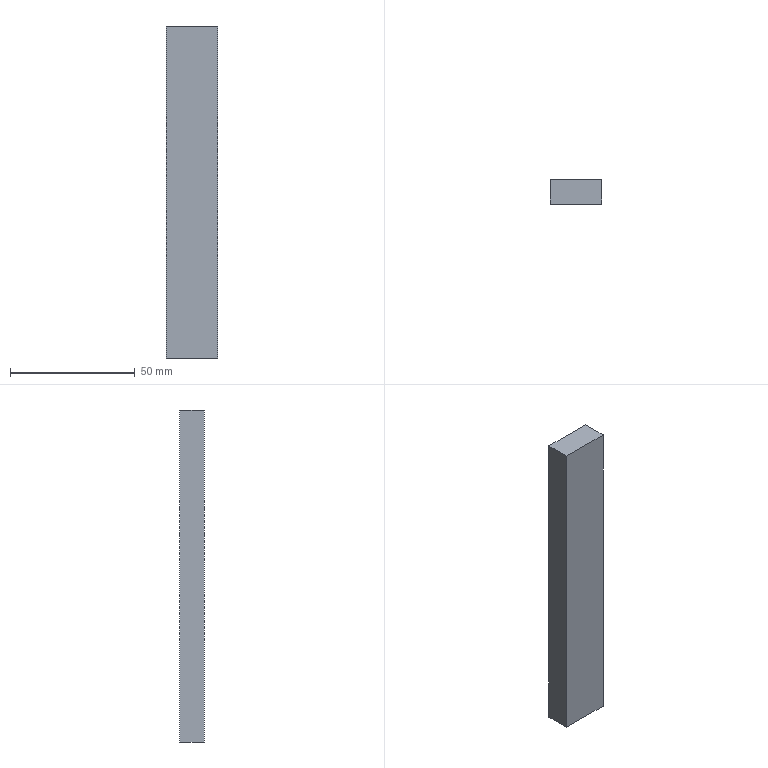Part | STEP file | 1 solid | 6 faces | box 20.737 x 10 x 133 mm | volume 27580 mm3 | plane 6
STEP:
#1=CARTESIAN_POINT('',(0.,0.,0.));
#2=DIRECTION('',(0.,0.,1.));
#3=DIRECTION('',(1.,0.,0.));
#4=AXIS2_PLACEMENT_3D('',#1,#2,#3);
#5=CARTESIAN_POINT('',(-23.708,79.267,216.926));
#6=VERTEX_POINT('',#5);
#7=CARTESIAN_POINT('',(-23.708,79.267,349.926));
#8=VERTEX_POINT('',#7);
#9=CARTESIAN_POINT('',(-23.708,79.267,216.926));
#10=DIRECTION('',(0.,0.,1.));
#11=VECTOR('',#10,1.);
#12=LINE('',#9,#11);
#13=CARTESIAN_POINT('',(-23.708,89.267,216.926));
#14=DIRECTION('',(1.,0.,0.));
#15=DIRECTION('',(0.,1.,0.));
#16=AXIS2_PLACEMENT_3D('',#13,#14,#15);
#17=PLANE('',#16);
#18=CARTESIAN_POINT('',(-10.,0.));
#19=DIRECTION('',(0.,1.));
#20=VECTOR('',#19,1.);
#21=LINE('',#18,#20);
#22=(GEOMETRIC_REPRESENTATION_CONTEXT(2)PARAMETRIC_REPRESENTATION_CONTEXT()REPRESENTATION_CONTEXT('',''));
#23=DEFINITIONAL_REPRESENTATION('',(#21),#22);
#24=PCURVE('',#17,#23);
#25=CARTESIAN_POINT('',(0.,79.267,0.));
#26=DIRECTION('',(0.,1.,0.));
#27=DIRECTION('',(0.,0.,1.));
#28=AXIS2_PLACEMENT_3D('',#25,#26,#27);
#29=PLANE('',#28);
#30=CARTESIAN_POINT('',(216.926,-23.708));
#31=DIRECTION('',(1.,0.));
#32=VECTOR('',#31,1.);
#33=LINE('',#30,#32);
#34=(GEOMETRIC_REPRESENTATION_CONTEXT(2)PARAMETRIC_REPRESENTATION_CONTEXT()REPRESENTATION_CONTEXT('',''));
#35=DEFINITIONAL_REPRESENTATION('',(#33),#34);
#36=PCURVE('',#29,#35);
#37=SURFACE_CURVE('',#12,(#24,#36),.PCURVE_S1.);
#38=EDGE_CURVE('',#6,#8,#37,.T.);
#39=ORIENTED_EDGE('',*,*,#38,.T.);
#40=CARTESIAN_POINT('',(-23.708,89.267,349.926));
#41=VERTEX_POINT('',#40);
#42=CARTESIAN_POINT('',(-23.708,89.267,349.926));
#43=DIRECTION('',(0.,-1.,0.));
#44=VECTOR('',#43,1.);
#45=LINE('',#42,#44);
#46=CARTESIAN_POINT('',(0.,133.));
#47=DIRECTION('',(-1.,0.));
#48=VECTOR('',#47,1.);
#49=LINE('',#46,#48);
#50=(GEOMETRIC_REPRESENTATION_CONTEXT(2)PARAMETRIC_REPRESENTATION_CONTEXT()REPRESENTATION_CONTEXT('',''));
#51=DEFINITIONAL_REPRESENTATION('',(#49),#50);
#52=PCURVE('',#17,#51);
#53=CARTESIAN_POINT('',(-23.708,89.267,349.926));
#54=DIRECTION('',(0.,0.,-1.));
#55=DIRECTION('',(-1.,0.,0.));
#56=AXIS2_PLACEMENT_3D('',#53,#54,#55);
#57=PLANE('',#56);
#58=CARTESIAN_POINT('',(0.,0.));
#59=DIRECTION('',(0.,-1.));
#60=VECTOR('',#59,1.);
#61=LINE('',#58,#60);
#62=(GEOMETRIC_REPRESENTATION_CONTEXT(2)PARAMETRIC_REPRESENTATION_CONTEXT()REPRESENTATION_CONTEXT('',''));
#63=DEFINITIONAL_REPRESENTATION('',(#61),#62);
#64=PCURVE('',#57,#63);
#65=SURFACE_CURVE('',#45,(#52,#64),.PCURVE_S1.);
#66=EDGE_CURVE('',#41,#8,#65,.T.);
#67=ORIENTED_EDGE('',*,*,#66,.F.);
#68=CARTESIAN_POINT('',(-23.708,89.267,216.926));
#69=VERTEX_POINT('',#68);
#70=CARTESIAN_POINT('',(-23.708,89.267,216.926));
#71=DIRECTION('',(0.,0.,1.));
#72=VECTOR('',#71,1.);
#73=LINE('',#70,#72);
#74=CARTESIAN_POINT('',(0.,0.));
#75=DIRECTION('',(0.,1.));
#76=VECTOR('',#75,1.);
#77=LINE('',#74,#76);
#78=(GEOMETRIC_REPRESENTATION_CONTEXT(2)PARAMETRIC_REPRESENTATION_CONTEXT()REPRESENTATION_CONTEXT('',''));
#79=DEFINITIONAL_REPRESENTATION('',(#77),#78);
#80=PCURVE('',#17,#79);
#81=CARTESIAN_POINT('',(0.,89.267,0.));
#82=DIRECTION('',(0.,1.,0.));
#83=DIRECTION('',(0.,0.,1.));
#84=AXIS2_PLACEMENT_3D('',#81,#82,#83);
#85=PLANE('',#84);
#86=CARTESIAN_POINT('',(216.926,-23.708));
#87=DIRECTION('',(1.,0.));
#88=VECTOR('',#87,1.);
#89=LINE('',#86,#88);
#90=(GEOMETRIC_REPRESENTATION_CONTEXT(2)PARAMETRIC_REPRESENTATION_CONTEXT()REPRESENTATION_CONTEXT('',''));
#91=DEFINITIONAL_REPRESENTATION('',(#89),#90);
#92=PCURVE('',#85,#91);
#93=SURFACE_CURVE('',#73,(#80,#92),.PCURVE_S1.);
#94=EDGE_CURVE('',#69,#41,#93,.T.);
#95=ORIENTED_EDGE('',*,*,#94,.F.);
#96=CARTESIAN_POINT('',(-23.708,89.267,216.926));
#97=DIRECTION('',(0.,-1.,0.));
#98=VECTOR('',#97,1.);
#99=LINE('',#96,#98);
#100=CARTESIAN_POINT('',(0.,0.));
#101=DIRECTION('',(-1.,0.));
#102=VECTOR('',#101,1.);
#103=LINE('',#100,#102);
#104=(GEOMETRIC_REPRESENTATION_CONTEXT(2)PARAMETRIC_REPRESENTATION_CONTEXT()REPRESENTATION_CONTEXT('',''));
#105=DEFINITIONAL_REPRESENTATION('',(#103),#104);
#106=PCURVE('',#17,#105);
#107=CARTESIAN_POINT('',(-23.708,89.267,216.926));
#108=DIRECTION('',(0.,0.,1.));
#109=DIRECTION('',(1.,0.,0.));
#110=AXIS2_PLACEMENT_3D('',#107,#108,#109);
#111=PLANE('',#110);
#112=CARTESIAN_POINT('',(0.,0.));
#113=DIRECTION('',(0.,-1.));
#114=VECTOR('',#113,1.);
#115=LINE('',#112,#114);
#116=(GEOMETRIC_REPRESENTATION_CONTEXT(2)PARAMETRIC_REPRESENTATION_CONTEXT()REPRESENTATION_CONTEXT('',''));
#117=DEFINITIONAL_REPRESENTATION('',(#115),#116);
#118=PCURVE('',#111,#117);
#119=SURFACE_CURVE('',#99,(#106,#118),.PCURVE_S1.);
#120=EDGE_CURVE('',#69,#6,#119,.T.);
#121=ORIENTED_EDGE('',*,*,#120,.T.);
#122=EDGE_LOOP('',(#39,#67,#95,#121));
#123=FACE_BOUND('',#122,.T.);
#124=ADVANCED_FACE('',(#123),#17,.F.);
#125=CARTESIAN_POINT('',(-2.971,79.267,349.926));
#126=VERTEX_POINT('',#125);
#127=CARTESIAN_POINT('',(-23.708,79.267,349.926));
#128=DIRECTION('',(1.,0.,0.));
#129=VECTOR('',#128,1.);
#130=LINE('',#127,#129);
#131=CARTESIAN_POINT('',(0.,-10.));
#132=DIRECTION('',(-1.,0.));
#133=VECTOR('',#132,1.);
#134=LINE('',#131,#133);
#135=(GEOMETRIC_REPRESENTATION_CONTEXT(2)PARAMETRIC_REPRESENTATION_CONTEXT()REPRESENTATION_CONTEXT('',''));
#136=DEFINITIONAL_REPRESENTATION('',(#134),#135);
#137=PCURVE('',#57,#136);
#138=CARTESIAN_POINT('',(349.926,-23.708));
#139=DIRECTION('',(0.,1.));
#140=VECTOR('',#139,1.);
#141=LINE('',#138,#140);
#142=(GEOMETRIC_REPRESENTATION_CONTEXT(2)PARAMETRIC_REPRESENTATION_CONTEXT()REPRESENTATION_CONTEXT('',''));
#143=DEFINITIONAL_REPRESENTATION('',(#141),#142);
#144=PCURVE('',#29,#143);
#145=SURFACE_CURVE('',#130,(#137,#144),.PCURVE_S1.);
#146=EDGE_CURVE('',#8,#126,#145,.T.);
#147=ORIENTED_EDGE('',*,*,#146,.T.);
#148=CARTESIAN_POINT('',(-2.971,89.267,349.926));
#149=VERTEX_POINT('',#148);
#150=CARTESIAN_POINT('',(-2.971,89.267,349.926));
#151=DIRECTION('',(0.,-1.,0.));
#152=VECTOR('',#151,1.);
#153=LINE('',#150,#152);
#154=CARTESIAN_POINT('',(-20.737,0.));
#155=DIRECTION('',(0.,-1.));
#156=VECTOR('',#155,1.);
#157=LINE('',#154,#156);
#158=(GEOMETRIC_REPRESENTATION_CONTEXT(2)PARAMETRIC_REPRESENTATION_CONTEXT()REPRESENTATION_CONTEXT('',''));
#159=DEFINITIONAL_REPRESENTATION('',(#157),#158);
#160=PCURVE('',#57,#159);
#161=CARTESIAN_POINT('',(-2.971,89.267,216.926));
#162=DIRECTION('',(-1.,0.,0.));
#163=DIRECTION('',(0.,0.,1.));
#164=AXIS2_PLACEMENT_3D('',#161,#162,#163);
#165=PLANE('',#164);
#166=CARTESIAN_POINT('',(133.,0.));
#167=DIRECTION('',(0.,-1.));
#168=VECTOR('',#167,1.);
#169=LINE('',#166,#168);
#170=(GEOMETRIC_REPRESENTATION_CONTEXT(2)PARAMETRIC_REPRESENTATION_CONTEXT()REPRESENTATION_CONTEXT('',''));
#171=DEFINITIONAL_REPRESENTATION('',(#169),#170);
#172=PCURVE('',#165,#171);
#173=SURFACE_CURVE('',#153,(#160,#172),.PCURVE_S1.);
#174=EDGE_CURVE('',#149,#126,#173,.T.);
#175=ORIENTED_EDGE('',*,*,#174,.F.);
#176=CARTESIAN_POINT('',(-23.708,89.267,349.926));
#177=DIRECTION('',(1.,0.,0.));
#178=VECTOR('',#177,1.);
#179=LINE('',#176,#178);
#180=CARTESIAN_POINT('',(0.,0.));
#181=DIRECTION('',(-1.,0.));
#182=VECTOR('',#181,1.);
#183=LINE('',#180,#182);
#184=(GEOMETRIC_REPRESENTATION_CONTEXT(2)PARAMETRIC_REPRESENTATION_CONTEXT()REPRESENTATION_CONTEXT('',''));
#185=DEFINITIONAL_REPRESENTATION('',(#183),#184);
#186=PCURVE('',#57,#185);
#187=CARTESIAN_POINT('',(349.926,-23.708));
#188=DIRECTION('',(0.,1.));
#189=VECTOR('',#188,1.);
#190=LINE('',#187,#189);
#191=(GEOMETRIC_REPRESENTATION_CONTEXT(2)PARAMETRIC_REPRESENTATION_CONTEXT()REPRESENTATION_CONTEXT('',''));
#192=DEFINITIONAL_REPRESENTATION('',(#190),#191);
#193=PCURVE('',#85,#192);
#194=SURFACE_CURVE('',#179,(#186,#193),.PCURVE_S1.);
#195=EDGE_CURVE('',#41,#149,#194,.T.);
#196=ORIENTED_EDGE('',*,*,#195,.F.);
#197=ORIENTED_EDGE('',*,*,#66,.T.);
#198=EDGE_LOOP('',(#147,#175,#196,#197));
#199=FACE_BOUND('',#198,.T.);
#200=ADVANCED_FACE('',(#199),#57,.F.);
#201=CARTESIAN_POINT('',(-2.971,79.267,216.926));
#202=VERTEX_POINT('',#201);
#203=CARTESIAN_POINT('',(-2.971,79.267,216.926));
#204=DIRECTION('',(0.,0.,-1.));
#205=VECTOR('',#204,1.);
#206=LINE('',#203,#205);
#207=CARTESIAN_POINT('',(0.,-10.));
#208=DIRECTION('',(-1.,0.));
#209=VECTOR('',#208,1.);
#210=LINE('',#207,#209);
#211=(GEOMETRIC_REPRESENTATION_CONTEXT(2)PARAMETRIC_REPRESENTATION_CONTEXT()REPRESENTATION_CONTEXT('',''));
#212=DEFINITIONAL_REPRESENTATION('',(#210),#211);
#213=PCURVE('',#165,#212);
#214=CARTESIAN_POINT('',(216.926,-2.971));
#215=DIRECTION('',(-1.,0.));
#216=VECTOR('',#215,1.);
#217=LINE('',#214,#216);
#218=(GEOMETRIC_REPRESENTATION_CONTEXT(2)PARAMETRIC_REPRESENTATION_CONTEXT()REPRESENTATION_CONTEXT('',''));
#219=DEFINITIONAL_REPRESENTATION('',(#217),#218);
#220=PCURVE('',#29,#219);
#221=SURFACE_CURVE('',#206,(#213,#220),.PCURVE_S1.);
#222=EDGE_CURVE('',#126,#202,#221,.T.);
#223=ORIENTED_EDGE('',*,*,#222,.T.);
#224=CARTESIAN_POINT('',(-2.971,89.267,216.926));
#225=VERTEX_POINT('',#224);
#226=CARTESIAN_POINT('',(-2.971,89.267,216.926));
#227=DIRECTION('',(0.,-1.,0.));
#228=VECTOR('',#227,1.);
#229=LINE('',#226,#228);
#230=CARTESIAN_POINT('',(0.,0.));
#231=DIRECTION('',(0.,-1.));
#232=VECTOR('',#231,1.);
#233=LINE('',#230,#232);
#234=(GEOMETRIC_REPRESENTATION_CONTEXT(2)PARAMETRIC_REPRESENTATION_CONTEXT()REPRESENTATION_CONTEXT('',''));
#235=DEFINITIONAL_REPRESENTATION('',(#233),#234);
#236=PCURVE('',#165,#235);
#237=CARTESIAN_POINT('',(20.737,0.));
#238=DIRECTION('',(0.,-1.));
#239=VECTOR('',#238,1.);
#240=LINE('',#237,#239);
#241=(GEOMETRIC_REPRESENTATION_CONTEXT(2)PARAMETRIC_REPRESENTATION_CONTEXT()REPRESENTATION_CONTEXT('',''));
#242=DEFINITIONAL_REPRESENTATION('',(#240),#241);
#243=PCURVE('',#111,#242);
#244=SURFACE_CURVE('',#229,(#236,#243),.PCURVE_S1.);
#245=EDGE_CURVE('',#225,#202,#244,.T.);
#246=ORIENTED_EDGE('',*,*,#245,.F.);
#247=CARTESIAN_POINT('',(-2.971,89.267,216.926));
#248=DIRECTION('',(0.,0.,-1.));
#249=VECTOR('',#248,1.);
#250=LINE('',#247,#249);
#251=CARTESIAN_POINT('',(0.,0.));
#252=DIRECTION('',(-1.,0.));
#253=VECTOR('',#252,1.);
#254=LINE('',#251,#253);
#255=(GEOMETRIC_REPRESENTATION_CONTEXT(2)PARAMETRIC_REPRESENTATION_CONTEXT()REPRESENTATION_CONTEXT('',''));
#256=DEFINITIONAL_REPRESENTATION('',(#254),#255);
#257=PCURVE('',#165,#256);
#258=CARTESIAN_POINT('',(216.926,-2.971));
#259=DIRECTION('',(-1.,0.));
#260=VECTOR('',#259,1.);
#261=LINE('',#258,#260);
#262=(GEOMETRIC_REPRESENTATION_CONTEXT(2)PARAMETRIC_REPRESENTATION_CONTEXT()REPRESENTATION_CONTEXT('',''));
#263=DEFINITIONAL_REPRESENTATION('',(#261),#262);
#264=PCURVE('',#85,#263);
#265=SURFACE_CURVE('',#250,(#257,#264),.PCURVE_S1.);
#266=EDGE_CURVE('',#149,#225,#265,.T.);
#267=ORIENTED_EDGE('',*,*,#266,.F.);
#268=ORIENTED_EDGE('',*,*,#174,.T.);
#269=EDGE_LOOP('',(#223,#246,#267,#268));
#270=FACE_BOUND('',#269,.T.);
#271=ADVANCED_FACE('',(#270),#165,.F.);
#272=CARTESIAN_POINT('',(-23.708,79.267,216.926));
#273=DIRECTION('',(-1.,0.,0.));
#274=VECTOR('',#273,1.);
#275=LINE('',#272,#274);
#276=CARTESIAN_POINT('',(0.,-10.));
#277=DIRECTION('',(-1.,0.));
#278=VECTOR('',#277,1.);
#279=LINE('',#276,#278);
#280=(GEOMETRIC_REPRESENTATION_CONTEXT(2)PARAMETRIC_REPRESENTATION_CONTEXT()REPRESENTATION_CONTEXT('',''));
#281=DEFINITIONAL_REPRESENTATION('',(#279),#280);
#282=PCURVE('',#111,#281);
#283=CARTESIAN_POINT('',(216.926,-23.708));
#284=DIRECTION('',(0.,-1.));
#285=VECTOR('',#284,1.);
#286=LINE('',#283,#285);
#287=(GEOMETRIC_REPRESENTATION_CONTEXT(2)PARAMETRIC_REPRESENTATION_CONTEXT()REPRESENTATION_CONTEXT('',''));
#288=DEFINITIONAL_REPRESENTATION('',(#286),#287);
#289=PCURVE('',#29,#288);
#290=SURFACE_CURVE('',#275,(#282,#289),.PCURVE_S1.);
#291=EDGE_CURVE('',#202,#6,#290,.T.);
#292=ORIENTED_EDGE('',*,*,#291,.T.);
#293=ORIENTED_EDGE('',*,*,#120,.F.);
#294=CARTESIAN_POINT('',(-23.708,89.267,216.926));
#295=DIRECTION('',(-1.,0.,0.));
#296=VECTOR('',#295,1.);
#297=LINE('',#294,#296);
#298=CARTESIAN_POINT('',(0.,0.));
#299=DIRECTION('',(-1.,0.));
#300=VECTOR('',#299,1.);
#301=LINE('',#298,#300);
#302=(GEOMETRIC_REPRESENTATION_CONTEXT(2)PARAMETRIC_REPRESENTATION_CONTEXT()REPRESENTATION_CONTEXT('',''));
#303=DEFINITIONAL_REPRESENTATION('',(#301),#302);
#304=PCURVE('',#111,#303);
#305=CARTESIAN_POINT('',(216.926,-23.708));
#306=DIRECTION('',(0.,-1.));
#307=VECTOR('',#306,1.);
#308=LINE('',#305,#307);
#309=(GEOMETRIC_REPRESENTATION_CONTEXT(2)PARAMETRIC_REPRESENTATION_CONTEXT()REPRESENTATION_CONTEXT('',''));
#310=DEFINITIONAL_REPRESENTATION('',(#308),#309);
#311=PCURVE('',#85,#310);
#312=SURFACE_CURVE('',#297,(#304,#311),.PCURVE_S1.);
#313=EDGE_CURVE('',#225,#69,#312,.T.);
#314=ORIENTED_EDGE('',*,*,#313,.F.);
#315=ORIENTED_EDGE('',*,*,#245,.T.);
#316=EDGE_LOOP('',(#292,#293,#314,#315));
#317=FACE_BOUND('',#316,.T.);
#318=ADVANCED_FACE('',(#317),#111,.F.);
#319=ORIENTED_EDGE('',*,*,#94,.T.);
#320=ORIENTED_EDGE('',*,*,#195,.T.);
#321=ORIENTED_EDGE('',*,*,#266,.T.);
#322=ORIENTED_EDGE('',*,*,#313,.T.);
#323=EDGE_LOOP('',(#319,#320,#321,#322));
#324=FACE_BOUND('',#323,.T.);
#325=ADVANCED_FACE('',(#324),#85,.T.);
#326=ORIENTED_EDGE('',*,*,#38,.F.);
#327=ORIENTED_EDGE('',*,*,#291,.F.);
#328=ORIENTED_EDGE('',*,*,#222,.F.);
#329=ORIENTED_EDGE('',*,*,#146,.F.);
#330=EDGE_LOOP('',(#326,#327,#328,#329));
#331=FACE_BOUND('',#330,.T.);
#332=ADVANCED_FACE('',(#331),#29,.F.);
#333=CLOSED_SHELL('',(#124,#200,#271,#318,#325,#332));
#334=MANIFOLD_SOLID_BREP('',#333);
#335=(LENGTH_UNIT()NAMED_UNIT(*)SI_UNIT(.MILLI.,.METRE.));
#336=UNCERTAINTY_MEASURE_WITH_UNIT(LENGTH_MEASURE(0.0000001),#335,'','');
#337=(NAMED_UNIT(*)PLANE_ANGLE_UNIT()SI_UNIT($,.RADIAN.));
#338=(NAMED_UNIT(*)SI_UNIT($,.STERADIAN.)SOLID_ANGLE_UNIT());
#339=(GEOMETRIC_REPRESENTATION_CONTEXT(3)GLOBAL_UNCERTAINTY_ASSIGNED_CONTEXT((#336))GLOBAL_UNIT_ASSIGNED_CONTEXT((#335,#337,#338))REPRESENTATION_CONTEXT('',''));
#340=ADVANCED_BREP_SHAPE_REPRESENTATION('',(#4,#334),#339);